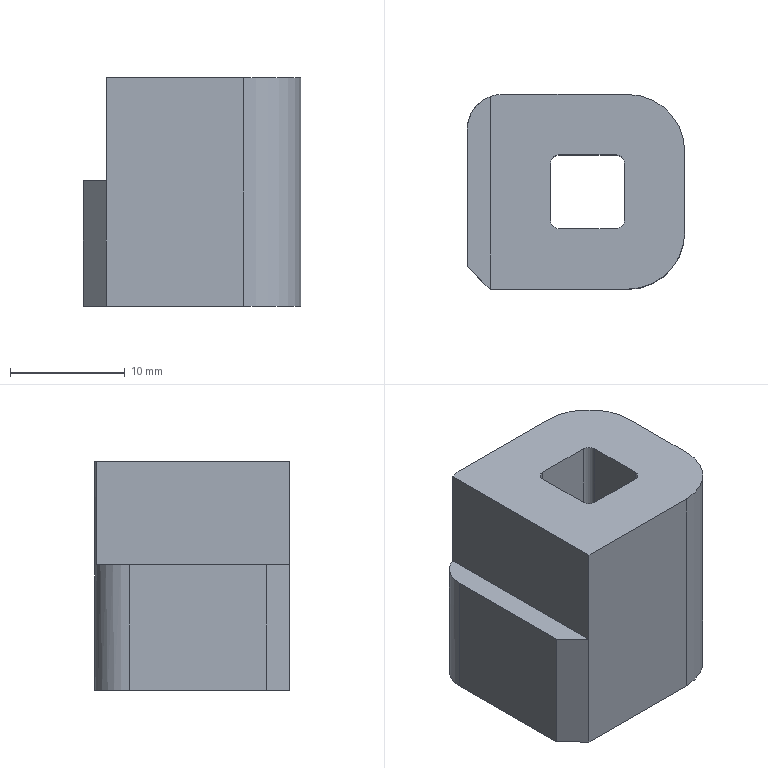Part | STEP file | 1 solid | 20 faces | box 19 x 17 x 20 mm | volume 5075 mm3 | plane 13 | cylinder 7 | commonest cylinder face diameters 1.44 x4 10 x2 6 x1
STEP:
#1=CARTESIAN_POINT('',(257.95,-38.262,-22.));
#2=VERTEX_POINT('',#1);
#3=CARTESIAN_POINT('',(269.95,-38.262,-22.));
#4=VERTEX_POINT('',#3);
#5=CARTESIAN_POINT('',(266.45,-38.262,-22.));
#6=DIRECTION('',(1.,0.,0.));
#7=VECTOR('',#6,1.);
#8=LINE('',#5,#7);
#9=EDGE_CURVE('',#2,#4,#8,.T.);
#10=ORIENTED_EDGE('',*,*,#9,.F.);
#11=CARTESIAN_POINT('',(255.95,-36.262,-22.));
#12=VERTEX_POINT('',#11);
#13=CARTESIAN_POINT('',(257.95,-38.262,-22.));
#14=DIRECTION('',(-0.7071,0.7071,0.));
#15=VECTOR('',#14,1.);
#16=LINE('',#13,#15);
#17=EDGE_CURVE('',#2,#12,#16,.T.);
#18=ORIENTED_EDGE('',*,*,#17,.T.);
#19=CARTESIAN_POINT('',(255.95,-24.262,-22.));
#20=VERTEX_POINT('',#19);
#21=CARTESIAN_POINT('',(255.95,-29.762,-22.));
#22=DIRECTION('',(0.,-1.,0.));
#23=VECTOR('',#22,1.);
#24=LINE('',#21,#23);
#25=EDGE_CURVE('',#20,#12,#24,.T.);
#26=ORIENTED_EDGE('',*,*,#25,.F.);
#27=CARTESIAN_POINT('',(258.95,-21.262,-22.));
#28=VERTEX_POINT('',#27);
#29=CARTESIAN_POINT('',(258.95,-24.262,-22.));
#30=DIRECTION('',(0.,0.,-1.));
#31=DIRECTION('',(-1.,0.,0.));
#32=AXIS2_PLACEMENT_3D('',#29,#30,#31);
#33=CIRCLE('',#32,3.);
#34=EDGE_CURVE('',#20,#28,#33,.T.);
#35=ORIENTED_EDGE('',*,*,#34,.T.);
#36=CARTESIAN_POINT('',(269.95,-21.262,-22.));
#37=VERTEX_POINT('',#36);
#38=CARTESIAN_POINT('',(266.45,-21.262,-22.));
#39=DIRECTION('',(-1.,0.,0.));
#40=VECTOR('',#39,1.);
#41=LINE('',#38,#40);
#42=EDGE_CURVE('',#37,#28,#41,.T.);
#43=ORIENTED_EDGE('',*,*,#42,.F.);
#44=CARTESIAN_POINT('',(274.95,-26.262,-22.));
#45=VERTEX_POINT('',#44);
#46=CARTESIAN_POINT('',(269.95,-26.262,-22.));
#47=DIRECTION('',(0.,0.,-1.));
#48=DIRECTION('',(-1.,0.,0.));
#49=AXIS2_PLACEMENT_3D('',#46,#47,#48);
#50=CIRCLE('',#49,5.);
#51=EDGE_CURVE('',#37,#45,#50,.T.);
#52=ORIENTED_EDGE('',*,*,#51,.T.);
#53=CARTESIAN_POINT('',(274.95,-33.262,-22.));
#54=VERTEX_POINT('',#53);
#55=CARTESIAN_POINT('',(274.95,-29.762,-22.));
#56=DIRECTION('',(0.,1.,0.));
#57=VECTOR('',#56,1.);
#58=LINE('',#55,#57);
#59=EDGE_CURVE('',#54,#45,#58,.T.);
#60=ORIENTED_EDGE('',*,*,#59,.F.);
#61=CARTESIAN_POINT('',(269.95,-33.262,-22.));
#62=DIRECTION('',(0.,0.,-1.));
#63=DIRECTION('',(-1.,0.,0.));
#64=AXIS2_PLACEMENT_3D('',#61,#62,#63);
#65=CIRCLE('',#64,5.);
#66=EDGE_CURVE('',#54,#4,#65,.T.);
#67=ORIENTED_EDGE('',*,*,#66,.T.);
#68=EDGE_LOOP('',(#10,#18,#26,#35,#43,#52,#60,#67));
#69=FACE_BOUND('',#68,.T.);
#70=CARTESIAN_POINT('',(263.23,-32.262,-22.));
#71=VERTEX_POINT('',#70);
#72=CARTESIAN_POINT('',(263.23,-27.262,-22.));
#73=VERTEX_POINT('',#72);
#74=CARTESIAN_POINT('',(263.23,-29.762,-22.));
#75=DIRECTION('',(0.,1.,0.));
#76=VECTOR('',#75,1.);
#77=LINE('',#74,#76);
#78=EDGE_CURVE('',#71,#73,#77,.T.);
#79=ORIENTED_EDGE('',*,*,#78,.F.);
#80=CARTESIAN_POINT('',(263.95,-32.982,-22.));
#81=VERTEX_POINT('',#80);
#82=CARTESIAN_POINT('',(263.95,-32.262,-22.));
#83=DIRECTION('',(0.,0.,-1.));
#84=DIRECTION('',(-1.,0.,0.));
#85=AXIS2_PLACEMENT_3D('',#82,#83,#84);
#86=CIRCLE('',#85,0.72);
#87=EDGE_CURVE('',#81,#71,#86,.T.);
#88=ORIENTED_EDGE('',*,*,#87,.F.);
#89=CARTESIAN_POINT('',(268.95,-32.982,-22.));
#90=VERTEX_POINT('',#89);
#91=CARTESIAN_POINT('',(268.95,-32.982,-22.));
#92=DIRECTION('',(1.,0.,0.));
#93=VECTOR('',#92,1.);
#94=LINE('',#91,#93);
#95=EDGE_CURVE('',#81,#90,#94,.T.);
#96=ORIENTED_EDGE('',*,*,#95,.T.);
#97=CARTESIAN_POINT('',(269.67,-32.262,-22.));
#98=VERTEX_POINT('',#97);
#99=CARTESIAN_POINT('',(268.95,-32.262,-22.));
#100=DIRECTION('',(0.,0.,1.));
#101=DIRECTION('',(-1.,0.,0.));
#102=AXIS2_PLACEMENT_3D('',#99,#100,#101);
#103=CIRCLE('',#102,0.72);
#104=EDGE_CURVE('',#90,#98,#103,.T.);
#105=ORIENTED_EDGE('',*,*,#104,.T.);
#106=CARTESIAN_POINT('',(269.67,-27.262,-22.));
#107=VERTEX_POINT('',#106);
#108=CARTESIAN_POINT('',(269.67,-29.762,-22.));
#109=DIRECTION('',(0.,-1.,0.));
#110=VECTOR('',#109,1.);
#111=LINE('',#108,#110);
#112=EDGE_CURVE('',#107,#98,#111,.T.);
#113=ORIENTED_EDGE('',*,*,#112,.F.);
#114=CARTESIAN_POINT('',(268.95,-26.542,-22.));
#115=VERTEX_POINT('',#114);
#116=CARTESIAN_POINT('',(268.95,-27.262,-22.));
#117=DIRECTION('',(0.,0.,-1.));
#118=DIRECTION('',(-1.,0.,0.));
#119=AXIS2_PLACEMENT_3D('',#116,#117,#118);
#120=CIRCLE('',#119,0.72);
#121=EDGE_CURVE('',#115,#107,#120,.T.);
#122=ORIENTED_EDGE('',*,*,#121,.F.);
#123=CARTESIAN_POINT('',(263.95,-26.542,-22.));
#124=VERTEX_POINT('',#123);
#125=CARTESIAN_POINT('',(266.45,-26.542,-22.));
#126=DIRECTION('',(1.,0.,0.));
#127=VECTOR('',#126,1.);
#128=LINE('',#125,#127);
#129=EDGE_CURVE('',#124,#115,#128,.T.);
#130=ORIENTED_EDGE('',*,*,#129,.F.);
#131=CARTESIAN_POINT('',(263.95,-27.262,-22.));
#132=DIRECTION('',(0.,0.,-1.));
#133=DIRECTION('',(-1.,0.,0.));
#134=AXIS2_PLACEMENT_3D('',#131,#132,#133);
#135=CIRCLE('',#134,0.72);
#136=EDGE_CURVE('',#73,#124,#135,.T.);
#137=ORIENTED_EDGE('',*,*,#136,.F.);
#138=EDGE_LOOP('',(#79,#88,#96,#105,#113,#122,#130,#137));
#139=FACE_BOUND('',#138,.T.);
#140=CARTESIAN_POINT('',(266.45,-29.762,-22.));
#141=DIRECTION('',(0.,0.,-1.));
#142=DIRECTION('',(-1.,0.,0.));
#143=AXIS2_PLACEMENT_3D('',#140,#141,#142);
#144=PLANE('',#143);
#145=ADVANCED_FACE('',(#69,#139),#144,.T.);
#146=CARTESIAN_POINT('',(269.67,-32.262,-2.));
#147=VERTEX_POINT('',#146);
#148=CARTESIAN_POINT('',(268.95,-32.982,-2.));
#149=VERTEX_POINT('',#148);
#150=CARTESIAN_POINT('',(268.95,-32.262,-2.));
#151=DIRECTION('',(0.,0.,-1.));
#152=DIRECTION('',(1.,0.,0.));
#153=AXIS2_PLACEMENT_3D('',#150,#151,#152);
#154=CIRCLE('',#153,0.72);
#155=EDGE_CURVE('',#147,#149,#154,.T.);
#156=ORIENTED_EDGE('',*,*,#155,.T.);
#157=CARTESIAN_POINT('',(263.95,-32.982,-2.));
#158=VERTEX_POINT('',#157);
#159=CARTESIAN_POINT('',(268.95,-32.982,-2.));
#160=DIRECTION('',(-1.,0.,0.));
#161=VECTOR('',#160,1.);
#162=LINE('',#159,#161);
#163=EDGE_CURVE('',#149,#158,#162,.T.);
#164=ORIENTED_EDGE('',*,*,#163,.T.);
#165=CARTESIAN_POINT('',(263.23,-32.262,-2.));
#166=VERTEX_POINT('',#165);
#167=CARTESIAN_POINT('',(263.95,-32.262,-2.));
#168=DIRECTION('',(0.,0.,-1.));
#169=DIRECTION('',(1.,0.,0.));
#170=AXIS2_PLACEMENT_3D('',#167,#168,#169);
#171=CIRCLE('',#170,0.72);
#172=EDGE_CURVE('',#158,#166,#171,.T.);
#173=ORIENTED_EDGE('',*,*,#172,.T.);
#174=CARTESIAN_POINT('',(263.23,-27.262,-2.));
#175=VERTEX_POINT('',#174);
#176=CARTESIAN_POINT('',(263.23,-32.262,-2.));
#177=DIRECTION('',(0.,1.,0.));
#178=VECTOR('',#177,1.);
#179=LINE('',#176,#178);
#180=EDGE_CURVE('',#166,#175,#179,.T.);
#181=ORIENTED_EDGE('',*,*,#180,.T.);
#182=CARTESIAN_POINT('',(263.95,-26.542,-2.));
#183=VERTEX_POINT('',#182);
#184=CARTESIAN_POINT('',(263.95,-27.262,-2.));
#185=DIRECTION('',(0.,0.,-1.));
#186=DIRECTION('',(1.,0.,0.));
#187=AXIS2_PLACEMENT_3D('',#184,#185,#186);
#188=CIRCLE('',#187,0.72);
#189=EDGE_CURVE('',#175,#183,#188,.T.);
#190=ORIENTED_EDGE('',*,*,#189,.T.);
#191=CARTESIAN_POINT('',(268.95,-26.542,-2.));
#192=VERTEX_POINT('',#191);
#193=CARTESIAN_POINT('',(263.95,-26.542,-2.));
#194=DIRECTION('',(1.,0.,0.));
#195=VECTOR('',#194,1.);
#196=LINE('',#193,#195);
#197=EDGE_CURVE('',#183,#192,#196,.T.);
#198=ORIENTED_EDGE('',*,*,#197,.T.);
#199=CARTESIAN_POINT('',(269.67,-27.262,-2.));
#200=VERTEX_POINT('',#199);
#201=CARTESIAN_POINT('',(268.95,-27.262,-2.));
#202=DIRECTION('',(0.,0.,-1.));
#203=DIRECTION('',(1.,0.,0.));
#204=AXIS2_PLACEMENT_3D('',#201,#202,#203);
#205=CIRCLE('',#204,0.72);
#206=EDGE_CURVE('',#192,#200,#205,.T.);
#207=ORIENTED_EDGE('',*,*,#206,.T.);
#208=CARTESIAN_POINT('',(269.67,-27.262,-2.));
#209=DIRECTION('',(0.,-1.,0.));
#210=VECTOR('',#209,1.);
#211=LINE('',#208,#210);
#212=EDGE_CURVE('',#200,#147,#211,.T.);
#213=ORIENTED_EDGE('',*,*,#212,.T.);
#214=EDGE_LOOP('',(#156,#164,#173,#181,#190,#198,#207,#213));
#215=FACE_BOUND('',#214,.T.);
#216=CARTESIAN_POINT('',(258.95,-21.262,-2.));
#217=VERTEX_POINT('',#216);
#218=CARTESIAN_POINT('',(269.95,-21.262,-2.));
#219=VERTEX_POINT('',#218);
#220=CARTESIAN_POINT('',(266.45,-21.262,-2.));
#221=DIRECTION('',(1.,0.,0.));
#222=VECTOR('',#221,1.);
#223=LINE('',#220,#222);
#224=EDGE_CURVE('',#217,#219,#223,.T.);
#225=ORIENTED_EDGE('',*,*,#224,.F.);
#226=CARTESIAN_POINT('',(257.95,-21.433,-2.));
#227=VERTEX_POINT('',#226);
#228=CARTESIAN_POINT('',(258.95,-24.262,-2.));
#229=DIRECTION('',(0.,0.,1.));
#230=DIRECTION('',(1.,0.,0.));
#231=AXIS2_PLACEMENT_3D('',#228,#229,#230);
#232=CIRCLE('',#231,3.);
#233=EDGE_CURVE('',#217,#227,#232,.T.);
#234=ORIENTED_EDGE('',*,*,#233,.T.);
#235=CARTESIAN_POINT('',(257.95,-38.262,-2.));
#236=VERTEX_POINT('',#235);
#237=CARTESIAN_POINT('',(257.95,-29.762,-2.));
#238=DIRECTION('',(0.,1.,0.));
#239=VECTOR('',#238,1.);
#240=LINE('',#237,#239);
#241=EDGE_CURVE('',#236,#227,#240,.T.);
#242=ORIENTED_EDGE('',*,*,#241,.F.);
#243=CARTESIAN_POINT('',(269.95,-38.262,-2.));
#244=VERTEX_POINT('',#243);
#245=CARTESIAN_POINT('',(266.45,-38.262,-2.));
#246=DIRECTION('',(-1.,0.,0.));
#247=VECTOR('',#246,1.);
#248=LINE('',#245,#247);
#249=EDGE_CURVE('',#244,#236,#248,.T.);
#250=ORIENTED_EDGE('',*,*,#249,.F.);
#251=CARTESIAN_POINT('',(274.95,-33.262,-2.));
#252=VERTEX_POINT('',#251);
#253=CARTESIAN_POINT('',(269.95,-33.262,-2.));
#254=DIRECTION('',(0.,0.,1.));
#255=DIRECTION('',(1.,0.,0.));
#256=AXIS2_PLACEMENT_3D('',#253,#254,#255);
#257=CIRCLE('',#256,5.);
#258=EDGE_CURVE('',#244,#252,#257,.T.);
#259=ORIENTED_EDGE('',*,*,#258,.T.);
#260=CARTESIAN_POINT('',(274.95,-26.262,-2.));
#261=VERTEX_POINT('',#260);
#262=CARTESIAN_POINT('',(274.95,-29.762,-2.));
#263=DIRECTION('',(0.,-1.,0.));
#264=VECTOR('',#263,1.);
#265=LINE('',#262,#264);
#266=EDGE_CURVE('',#261,#252,#265,.T.);
#267=ORIENTED_EDGE('',*,*,#266,.F.);
#268=CARTESIAN_POINT('',(269.95,-26.262,-2.));
#269=DIRECTION('',(0.,0.,1.));
#270=DIRECTION('',(1.,0.,0.));
#271=AXIS2_PLACEMENT_3D('',#268,#269,#270);
#272=CIRCLE('',#271,5.);
#273=EDGE_CURVE('',#261,#219,#272,.T.);
#274=ORIENTED_EDGE('',*,*,#273,.T.);
#275=EDGE_LOOP('',(#225,#234,#242,#250,#259,#267,#274));
#276=FACE_BOUND('',#275,.T.);
#277=CARTESIAN_POINT('',(266.45,-29.762,-2.));
#278=DIRECTION('',(0.,0.,1.));
#279=DIRECTION('',(1.,0.,0.));
#280=AXIS2_PLACEMENT_3D('',#277,#278,#279);
#281=PLANE('',#280);
#282=ADVANCED_FACE('',(#215,#276),#281,.T.);
#283=CARTESIAN_POINT('',(257.95,-38.262,-11.));
#284=VERTEX_POINT('',#283);
#285=CARTESIAN_POINT('',(257.95,-38.262,-22.));
#286=DIRECTION('',(0.,0.,1.));
#287=VECTOR('',#286,1.);
#288=LINE('',#285,#287);
#289=EDGE_CURVE('',#284,#236,#288,.T.);
#290=ORIENTED_EDGE('',*,*,#289,.F.);
#291=CARTESIAN_POINT('',(257.95,-38.262,-22.));
#292=DIRECTION('',(0.,0.,-1.));
#293=VECTOR('',#292,1.);
#294=LINE('',#291,#293);
#295=EDGE_CURVE('',#284,#2,#294,.T.);
#296=ORIENTED_EDGE('',*,*,#295,.T.);
#297=ORIENTED_EDGE('',*,*,#9,.T.);
#298=CARTESIAN_POINT('',(269.95,-38.262,-22.));
#299=DIRECTION('',(0.,0.,1.));
#300=VECTOR('',#299,1.);
#301=LINE('',#298,#300);
#302=EDGE_CURVE('',#4,#244,#301,.T.);
#303=ORIENTED_EDGE('',*,*,#302,.T.);
#304=ORIENTED_EDGE('',*,*,#249,.T.);
#305=EDGE_LOOP('',(#290,#296,#297,#303,#304));
#306=FACE_OUTER_BOUND('',#305,.T.);
#307=CARTESIAN_POINT('',(266.45,-38.262,-22.));
#308=DIRECTION('',(0.,-1.,0.));
#309=DIRECTION('',(0.,0.,-1.));
#310=AXIS2_PLACEMENT_3D('',#307,#308,#309);
#311=PLANE('',#310);
#312=ADVANCED_FACE('',(#306),#311,.T.);
#313=ORIENTED_EDGE('',*,*,#241,.T.);
#314=CARTESIAN_POINT('',(257.95,-21.433,-11.));
#315=VERTEX_POINT('',#314);
#316=CARTESIAN_POINT('',(257.95,-21.433,-2.));
#317=DIRECTION('',(0.,0.,-1.));
#318=VECTOR('',#317,1.);
#319=LINE('',#316,#318);
#320=EDGE_CURVE('',#227,#315,#319,.T.);
#321=ORIENTED_EDGE('',*,*,#320,.T.);
#322=CARTESIAN_POINT('',(257.95,-29.762,-11.));
#323=DIRECTION('',(0.,1.,0.));
#324=VECTOR('',#323,1.);
#325=LINE('',#322,#324);
#326=EDGE_CURVE('',#284,#315,#325,.T.);
#327=ORIENTED_EDGE('',*,*,#326,.F.);
#328=ORIENTED_EDGE('',*,*,#289,.T.);
#329=EDGE_LOOP('',(#313,#321,#327,#328));
#330=FACE_OUTER_BOUND('',#329,.T.);
#331=CARTESIAN_POINT('',(257.95,-29.762,-22.));
#332=DIRECTION('',(-1.,0.,0.));
#333=DIRECTION('',(0.,0.,1.));
#334=AXIS2_PLACEMENT_3D('',#331,#332,#333);
#335=PLANE('',#334);
#336=ADVANCED_FACE('',(#330),#335,.T.);
#337=ORIENTED_EDGE('',*,*,#42,.T.);
#338=CARTESIAN_POINT('',(258.95,-21.262,-22.));
#339=DIRECTION('',(0.,0.,1.));
#340=VECTOR('',#339,1.);
#341=LINE('',#338,#340);
#342=EDGE_CURVE('',#28,#217,#341,.T.);
#343=ORIENTED_EDGE('',*,*,#342,.T.);
#344=ORIENTED_EDGE('',*,*,#224,.T.);
#345=CARTESIAN_POINT('',(269.95,-21.262,-22.));
#346=DIRECTION('',(0.,0.,-1.));
#347=VECTOR('',#346,1.);
#348=LINE('',#345,#347);
#349=EDGE_CURVE('',#219,#37,#348,.T.);
#350=ORIENTED_EDGE('',*,*,#349,.T.);
#351=EDGE_LOOP('',(#337,#343,#344,#350));
#352=FACE_OUTER_BOUND('',#351,.T.);
#353=CARTESIAN_POINT('',(266.45,-21.262,-22.));
#354=DIRECTION('',(0.,1.,0.));
#355=DIRECTION('',(0.,0.,1.));
#356=AXIS2_PLACEMENT_3D('',#353,#354,#355);
#357=PLANE('',#356);
#358=ADVANCED_FACE('',(#352),#357,.T.);
#359=ORIENTED_EDGE('',*,*,#266,.T.);
#360=CARTESIAN_POINT('',(274.95,-33.262,-22.));
#361=DIRECTION('',(0.,0.,-1.));
#362=VECTOR('',#361,1.);
#363=LINE('',#360,#362);
#364=EDGE_CURVE('',#252,#54,#363,.T.);
#365=ORIENTED_EDGE('',*,*,#364,.T.);
#366=ORIENTED_EDGE('',*,*,#59,.T.);
#367=CARTESIAN_POINT('',(274.95,-26.262,-22.));
#368=DIRECTION('',(0.,0.,1.));
#369=VECTOR('',#368,1.);
#370=LINE('',#367,#369);
#371=EDGE_CURVE('',#45,#261,#370,.T.);
#372=ORIENTED_EDGE('',*,*,#371,.T.);
#373=EDGE_LOOP('',(#359,#365,#366,#372));
#374=FACE_OUTER_BOUND('',#373,.T.);
#375=CARTESIAN_POINT('',(274.95,-29.762,-22.));
#376=DIRECTION('',(1.,0.,0.));
#377=DIRECTION('',(0.,0.,-1.));
#378=AXIS2_PLACEMENT_3D('',#375,#376,#377);
#379=PLANE('',#378);
#380=ADVANCED_FACE('',(#374),#379,.T.);
#381=CARTESIAN_POINT('',(255.95,-36.262,-11.));
#382=VERTEX_POINT('',#381);
#383=CARTESIAN_POINT('',(255.95,-24.262,-11.));
#384=VERTEX_POINT('',#383);
#385=CARTESIAN_POINT('',(255.95,-29.762,-11.));
#386=DIRECTION('',(0.,1.,0.));
#387=VECTOR('',#386,1.);
#388=LINE('',#385,#387);
#389=EDGE_CURVE('',#382,#384,#388,.T.);
#390=ORIENTED_EDGE('',*,*,#389,.F.);
#391=CARTESIAN_POINT('',(255.95,-36.262,-11.));
#392=DIRECTION('',(0.7071,-0.7071,0.));
#393=VECTOR('',#392,1.);
#394=LINE('',#391,#393);
#395=EDGE_CURVE('',#382,#284,#394,.T.);
#396=ORIENTED_EDGE('',*,*,#395,.T.);
#397=ORIENTED_EDGE('',*,*,#326,.T.);
#398=CARTESIAN_POINT('',(258.95,-24.262,-11.));
#399=DIRECTION('',(0.,0.,1.));
#400=DIRECTION('',(1.,0.,0.));
#401=AXIS2_PLACEMENT_3D('',#398,#399,#400);
#402=CIRCLE('',#401,3.);
#403=EDGE_CURVE('',#315,#384,#402,.T.);
#404=ORIENTED_EDGE('',*,*,#403,.T.);
#405=EDGE_LOOP('',(#390,#396,#397,#404));
#406=FACE_OUTER_BOUND('',#405,.T.);
#407=CARTESIAN_POINT('',(259.95,-29.762,-11.));
#408=DIRECTION('',(0.,0.,1.));
#409=DIRECTION('',(0.,1.,0.));
#410=AXIS2_PLACEMENT_3D('',#407,#408,#409);
#411=PLANE('',#410);
#412=ADVANCED_FACE('',(#406),#411,.T.);
#413=ORIENTED_EDGE('',*,*,#25,.T.);
#414=CARTESIAN_POINT('',(255.95,-36.262,-22.));
#415=DIRECTION('',(0.,0.,1.));
#416=VECTOR('',#415,1.);
#417=LINE('',#414,#416);
#418=EDGE_CURVE('',#12,#382,#417,.T.);
#419=ORIENTED_EDGE('',*,*,#418,.T.);
#420=ORIENTED_EDGE('',*,*,#389,.T.);
#421=CARTESIAN_POINT('',(255.95,-24.262,-22.));
#422=DIRECTION('',(0.,0.,-1.));
#423=VECTOR('',#422,1.);
#424=LINE('',#421,#423);
#425=EDGE_CURVE('',#384,#20,#424,.T.);
#426=ORIENTED_EDGE('',*,*,#425,.T.);
#427=EDGE_LOOP('',(#413,#419,#420,#426));
#428=FACE_OUTER_BOUND('',#427,.T.);
#429=CARTESIAN_POINT('',(255.95,-29.762,-22.));
#430=DIRECTION('',(-1.,0.,0.));
#431=DIRECTION('',(0.,0.,1.));
#432=AXIS2_PLACEMENT_3D('',#429,#430,#431);
#433=PLANE('',#432);
#434=ADVANCED_FACE('',(#428),#433,.T.);
#435=CARTESIAN_POINT('',(268.95,-32.982,71.));
#436=DIRECTION('',(0.,0.,1.));
#437=VECTOR('',#436,1.);
#438=LINE('',#435,#437);
#439=EDGE_CURVE('',#90,#149,#438,.T.);
#440=ORIENTED_EDGE('',*,*,#439,.T.);
#441=ORIENTED_EDGE('',*,*,#155,.F.);
#442=CARTESIAN_POINT('',(269.67,-32.262,71.));
#443=DIRECTION('',(0.,0.,1.));
#444=VECTOR('',#443,1.);
#445=LINE('',#442,#444);
#446=EDGE_CURVE('',#98,#147,#445,.T.);
#447=ORIENTED_EDGE('',*,*,#446,.F.);
#448=ORIENTED_EDGE('',*,*,#104,.F.);
#449=EDGE_LOOP('',(#440,#441,#447,#448));
#450=FACE_OUTER_BOUND('',#449,.T.);
#451=CARTESIAN_POINT('',(268.95,-32.262,71.));
#452=DIRECTION('',(0.,0.,-1.));
#453=DIRECTION('',(-1.,0.,0.));
#454=AXIS2_PLACEMENT_3D('',#451,#452,#453);
#455=CYLINDRICAL_SURFACE('',#454,0.72);
#456=ADVANCED_FACE('',(#450),#455,.F.);
#457=ORIENTED_EDGE('',*,*,#446,.T.);
#458=ORIENTED_EDGE('',*,*,#212,.F.);
#459=CARTESIAN_POINT('',(269.67,-27.262,71.));
#460=DIRECTION('',(0.,0.,1.));
#461=VECTOR('',#460,1.);
#462=LINE('',#459,#461);
#463=EDGE_CURVE('',#107,#200,#462,.T.);
#464=ORIENTED_EDGE('',*,*,#463,.F.);
#465=ORIENTED_EDGE('',*,*,#112,.T.);
#466=EDGE_LOOP('',(#457,#458,#464,#465));
#467=FACE_OUTER_BOUND('',#466,.T.);
#468=CARTESIAN_POINT('',(269.67,-27.262,71.));
#469=DIRECTION('',(1.,0.,0.));
#470=DIRECTION('',(0.,0.,-1.));
#471=AXIS2_PLACEMENT_3D('',#468,#469,#470);
#472=PLANE('',#471);
#473=ADVANCED_FACE('',(#467),#472,.F.);
#474=ORIENTED_EDGE('',*,*,#463,.T.);
#475=ORIENTED_EDGE('',*,*,#206,.F.);
#476=CARTESIAN_POINT('',(268.95,-26.542,71.));
#477=DIRECTION('',(0.,0.,1.));
#478=VECTOR('',#477,1.);
#479=LINE('',#476,#478);
#480=EDGE_CURVE('',#115,#192,#479,.T.);
#481=ORIENTED_EDGE('',*,*,#480,.F.);
#482=ORIENTED_EDGE('',*,*,#121,.T.);
#483=EDGE_LOOP('',(#474,#475,#481,#482));
#484=FACE_OUTER_BOUND('',#483,.T.);
#485=CARTESIAN_POINT('',(268.95,-27.262,71.));
#486=DIRECTION('',(0.,0.,-1.));
#487=DIRECTION('',(-1.,0.,0.));
#488=AXIS2_PLACEMENT_3D('',#485,#486,#487);
#489=CYLINDRICAL_SURFACE('',#488,0.72);
#490=ADVANCED_FACE('',(#484),#489,.F.);
#491=ORIENTED_EDGE('',*,*,#480,.T.);
#492=ORIENTED_EDGE('',*,*,#197,.F.);
#493=CARTESIAN_POINT('',(263.95,-26.542,71.));
#494=DIRECTION('',(0.,0.,1.));
#495=VECTOR('',#494,1.);
#496=LINE('',#493,#495);
#497=EDGE_CURVE('',#124,#183,#496,.T.);
#498=ORIENTED_EDGE('',*,*,#497,.F.);
#499=ORIENTED_EDGE('',*,*,#129,.T.);
#500=EDGE_LOOP('',(#491,#492,#498,#499));
#501=FACE_OUTER_BOUND('',#500,.T.);
#502=CARTESIAN_POINT('',(263.95,-26.542,71.));
#503=DIRECTION('',(0.,1.,0.));
#504=DIRECTION('',(-1.,0.,0.));
#505=AXIS2_PLACEMENT_3D('',#502,#503,#504);
#506=PLANE('',#505);
#507=ADVANCED_FACE('',(#501),#506,.F.);
#508=ORIENTED_EDGE('',*,*,#497,.T.);
#509=ORIENTED_EDGE('',*,*,#189,.F.);
#510=CARTESIAN_POINT('',(263.23,-27.262,71.));
#511=DIRECTION('',(0.,0.,1.));
#512=VECTOR('',#511,1.);
#513=LINE('',#510,#512);
#514=EDGE_CURVE('',#73,#175,#513,.T.);
#515=ORIENTED_EDGE('',*,*,#514,.F.);
#516=ORIENTED_EDGE('',*,*,#136,.T.);
#517=EDGE_LOOP('',(#508,#509,#515,#516));
#518=FACE_OUTER_BOUND('',#517,.T.);
#519=CARTESIAN_POINT('',(263.95,-27.262,71.));
#520=DIRECTION('',(0.,0.,-1.));
#521=DIRECTION('',(-1.,0.,0.));
#522=AXIS2_PLACEMENT_3D('',#519,#520,#521);
#523=CYLINDRICAL_SURFACE('',#522,0.72);
#524=ADVANCED_FACE('',(#518),#523,.F.);
#525=ORIENTED_EDGE('',*,*,#514,.T.);
#526=ORIENTED_EDGE('',*,*,#180,.F.);
#527=CARTESIAN_POINT('',(263.23,-32.262,71.));
#528=DIRECTION('',(0.,0.,1.));
#529=VECTOR('',#528,1.);
#530=LINE('',#527,#529);
#531=EDGE_CURVE('',#71,#166,#530,.T.);
#532=ORIENTED_EDGE('',*,*,#531,.F.);
#533=ORIENTED_EDGE('',*,*,#78,.T.);
#534=EDGE_LOOP('',(#525,#526,#532,#533));
#535=FACE_OUTER_BOUND('',#534,.T.);
#536=CARTESIAN_POINT('',(263.23,-32.262,71.));
#537=DIRECTION('',(-1.,0.,0.));
#538=DIRECTION('',(0.,0.,1.));
#539=AXIS2_PLACEMENT_3D('',#536,#537,#538);
#540=PLANE('',#539);
#541=ADVANCED_FACE('',(#535),#540,.F.);
#542=ORIENTED_EDGE('',*,*,#531,.T.);
#543=ORIENTED_EDGE('',*,*,#172,.F.);
#544=CARTESIAN_POINT('',(263.95,-32.982,71.));
#545=DIRECTION('',(0.,0.,1.));
#546=VECTOR('',#545,1.);
#547=LINE('',#544,#546);
#548=EDGE_CURVE('',#81,#158,#547,.T.);
#549=ORIENTED_EDGE('',*,*,#548,.F.);
#550=ORIENTED_EDGE('',*,*,#87,.T.);
#551=EDGE_LOOP('',(#542,#543,#549,#550));
#552=FACE_OUTER_BOUND('',#551,.T.);
#553=CARTESIAN_POINT('',(263.95,-32.262,71.));
#554=DIRECTION('',(0.,0.,-1.));
#555=DIRECTION('',(-1.,0.,0.));
#556=AXIS2_PLACEMENT_3D('',#553,#554,#555);
#557=CYLINDRICAL_SURFACE('',#556,0.72);
#558=ADVANCED_FACE('',(#552),#557,.F.);
#559=ORIENTED_EDGE('',*,*,#548,.T.);
#560=ORIENTED_EDGE('',*,*,#163,.F.);
#561=ORIENTED_EDGE('',*,*,#439,.F.);
#562=ORIENTED_EDGE('',*,*,#95,.F.);
#563=EDGE_LOOP('',(#559,#560,#561,#562));
#564=FACE_OUTER_BOUND('',#563,.T.);
#565=CARTESIAN_POINT('',(268.95,-32.982,71.));
#566=DIRECTION('',(0.,-1.,0.));
#567=DIRECTION('',(0.,0.,-1.));
#568=AXIS2_PLACEMENT_3D('',#565,#566,#567);
#569=PLANE('',#568);
#570=ADVANCED_FACE('',(#564),#569,.F.);
#571=ORIENTED_EDGE('',*,*,#66,.F.);
#572=ORIENTED_EDGE('',*,*,#364,.F.);
#573=ORIENTED_EDGE('',*,*,#258,.F.);
#574=ORIENTED_EDGE('',*,*,#302,.F.);
#575=EDGE_LOOP('',(#571,#572,#573,#574));
#576=FACE_OUTER_BOUND('',#575,.T.);
#577=CARTESIAN_POINT('',(269.95,-33.262,-22.));
#578=DIRECTION('',(0.,0.,1.));
#579=DIRECTION('',(1.,0.,0.));
#580=AXIS2_PLACEMENT_3D('',#577,#578,#579);
#581=CYLINDRICAL_SURFACE('',#580,5.);
#582=ADVANCED_FACE('',(#576),#581,.T.);
#583=ORIENTED_EDGE('',*,*,#51,.F.);
#584=ORIENTED_EDGE('',*,*,#349,.F.);
#585=ORIENTED_EDGE('',*,*,#273,.F.);
#586=ORIENTED_EDGE('',*,*,#371,.F.);
#587=EDGE_LOOP('',(#583,#584,#585,#586));
#588=FACE_OUTER_BOUND('',#587,.T.);
#589=CARTESIAN_POINT('',(269.95,-26.262,-22.));
#590=DIRECTION('',(0.,0.,1.));
#591=DIRECTION('',(1.,0.,0.));
#592=AXIS2_PLACEMENT_3D('',#589,#590,#591);
#593=CYLINDRICAL_SURFACE('',#592,5.);
#594=ADVANCED_FACE('',(#588),#593,.T.);
#595=ORIENTED_EDGE('',*,*,#34,.F.);
#596=ORIENTED_EDGE('',*,*,#425,.F.);
#597=ORIENTED_EDGE('',*,*,#403,.F.);
#598=ORIENTED_EDGE('',*,*,#320,.F.);
#599=ORIENTED_EDGE('',*,*,#233,.F.);
#600=ORIENTED_EDGE('',*,*,#342,.F.);
#601=EDGE_LOOP('',(#595,#596,#597,#598,#599,#600));
#602=FACE_OUTER_BOUND('',#601,.T.);
#603=CARTESIAN_POINT('',(258.95,-24.262,-22.));
#604=DIRECTION('',(0.,0.,1.));
#605=DIRECTION('',(1.,0.,0.));
#606=AXIS2_PLACEMENT_3D('',#603,#604,#605);
#607=CYLINDRICAL_SURFACE('',#606,3.);
#608=ADVANCED_FACE('',(#602),#607,.T.);
#609=ORIENTED_EDGE('',*,*,#17,.F.);
#610=ORIENTED_EDGE('',*,*,#295,.F.);
#611=ORIENTED_EDGE('',*,*,#395,.F.);
#612=ORIENTED_EDGE('',*,*,#418,.F.);
#613=EDGE_LOOP('',(#609,#610,#611,#612));
#614=FACE_OUTER_BOUND('',#613,.T.);
#615=CARTESIAN_POINT('',(255.95,-36.262,-22.));
#616=DIRECTION('',(0.7071,0.7071,0.));
#617=DIRECTION('',(0.,0.,1.));
#618=AXIS2_PLACEMENT_3D('',#615,#616,#617);
#619=PLANE('',#618);
#620=ADVANCED_FACE('',(#614),#619,.F.);
#621=CLOSED_SHELL('',(#145,#282,#312,#336,#358,#380,#412,#434,#456,#473,#490,#507,#524,#541,#558,#570,#582,#594,#608,#620));
#622=MANIFOLD_SOLID_BREP('',#621);
#623=(LENGTH_UNIT()NAMED_UNIT(*)SI_UNIT(.MILLI.,.METRE.));
#624=UNCERTAINTY_MEASURE_WITH_UNIT(LENGTH_MEASURE(0.00002),#623,'','');
#625=(NAMED_UNIT(*)PLANE_ANGLE_UNIT()SI_UNIT($,.RADIAN.));
#626=PLANE_ANGLE_MEASURE_WITH_UNIT(PLANE_ANGLE_MEASURE(0.01745),#625);
#627=DIMENSIONAL_EXPONENTS(0.,0.,0.,0.,0.,0.,0.);
#628=(CONVERSION_BASED_UNIT('DEGREE',#626)NAMED_UNIT(#627)PLANE_ANGLE_UNIT());
#629=(NAMED_UNIT(*)SI_UNIT($,.STERADIAN.)SOLID_ANGLE_UNIT());
#630=(GEOMETRIC_REPRESENTATION_CONTEXT(3)GLOBAL_UNCERTAINTY_ASSIGNED_CONTEXT((#624))GLOBAL_UNIT_ASSIGNED_CONTEXT((#623,#628,#629))REPRESENTATION_CONTEXT('',''));
#631=ADVANCED_BREP_SHAPE_REPRESENTATION('',(#622),#630);